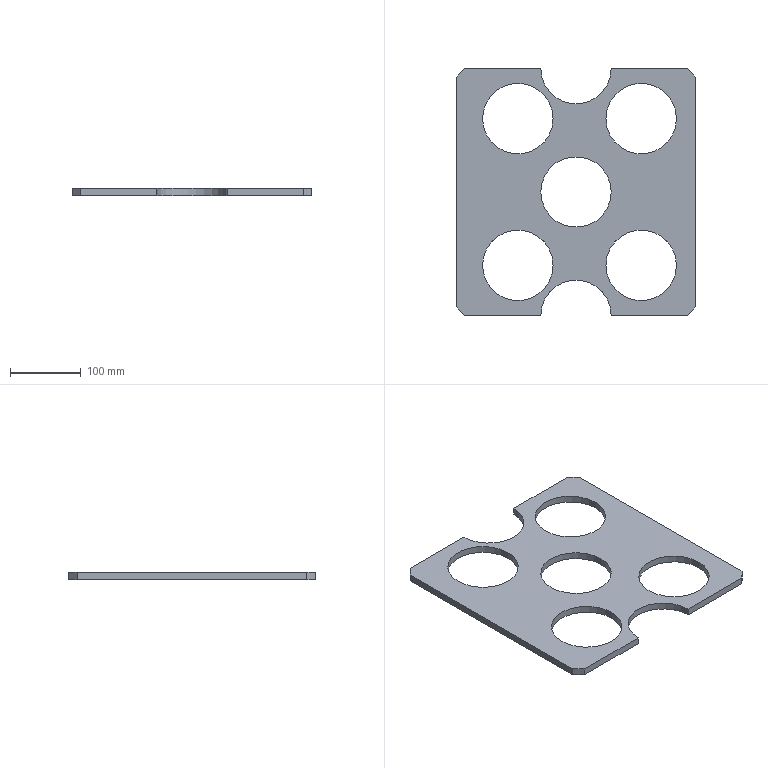Part | SolidWorks | features Extrusion 1 | 1 solid | 24 faces | box 340 x 350 x 10 mm | volume 715881 mm3 | cylinder 12 | plane 12 | commonest cylinder face diameters 100 x12
STEP:
#1=CARTESIAN_POINT('',(212.5,71.,10.));
#2=VERTEX_POINT('',#1);
#3=CARTESIAN_POINT('',(312.5,71.,10.));
#4=VERTEX_POINT('',#3);
#5=CARTESIAN_POINT('',(262.5,71.,10.));
#6=DIRECTION('',(0.,0.,1.));
#7=DIRECTION('',(-1.,0.,0.));
#8=AXIS2_PLACEMENT_3D('',#5,#6,#7);
#9=CIRCLE('',#8,50.);
#10=EDGE_CURVE('',#2,#4,#9,.T.);
#11=ORIENTED_EDGE('',*,*,#10,.T.);
#12=CARTESIAN_POINT('',(312.5,71.,0.));
#13=VERTEX_POINT('',#12);
#14=CARTESIAN_POINT('',(312.5,71.,10.));
#15=DIRECTION('',(0.,0.,-1.));
#16=VECTOR('',#15,1000.);
#17=LINE('',#14,#16);
#18=EDGE_CURVE('',#4,#13,#17,.T.);
#19=ORIENTED_EDGE('',*,*,#18,.T.);
#20=CARTESIAN_POINT('',(212.5,71.,0.));
#21=VERTEX_POINT('',#20);
#22=CARTESIAN_POINT('',(262.5,71.,0.));
#23=DIRECTION('',(0.,0.,1.));
#24=DIRECTION('',(-1.,0.,0.));
#25=AXIS2_PLACEMENT_3D('',#22,#23,#24);
#26=CIRCLE('',#25,50.);
#27=EDGE_CURVE('',#21,#13,#26,.T.);
#28=ORIENTED_EDGE('',*,*,#27,.F.);
#29=CARTESIAN_POINT('',(212.5,71.,10.));
#30=DIRECTION('',(0.,0.,-1.));
#31=VECTOR('',#30,1000.);
#32=LINE('',#29,#31);
#33=EDGE_CURVE('',#2,#21,#32,.T.);
#34=ORIENTED_EDGE('',*,*,#33,.F.);
#35=EDGE_LOOP('',(#11,#19,#28,#34));
#36=FACE_OUTER_BOUND('',#35,.T.);
#37=CARTESIAN_POINT('',(262.5,71.,10.));
#38=DIRECTION('',(0.,0.,-1.));
#39=DIRECTION('',(-1.,0.,0.));
#40=AXIS2_PLACEMENT_3D('',#37,#38,#39);
#41=CYLINDRICAL_SURFACE('',#40,50.);
#42=ADVANCED_FACE('',(#36),#41,.F.);
#43=CARTESIAN_POINT('',(37.5,71.,10.));
#44=VERTEX_POINT('',#43);
#45=CARTESIAN_POINT('',(137.5,71.,10.));
#46=VERTEX_POINT('',#45);
#47=CARTESIAN_POINT('',(87.5,71.,10.));
#48=DIRECTION('',(0.,0.,1.));
#49=DIRECTION('',(-1.,0.,0.));
#50=AXIS2_PLACEMENT_3D('',#47,#48,#49);
#51=CIRCLE('',#50,50.);
#52=EDGE_CURVE('',#44,#46,#51,.T.);
#53=ORIENTED_EDGE('',*,*,#52,.T.);
#54=CARTESIAN_POINT('',(137.5,71.,0.));
#55=VERTEX_POINT('',#54);
#56=CARTESIAN_POINT('',(137.5,71.,10.));
#57=DIRECTION('',(0.,0.,-1.));
#58=VECTOR('',#57,1000.);
#59=LINE('',#56,#58);
#60=EDGE_CURVE('',#46,#55,#59,.T.);
#61=ORIENTED_EDGE('',*,*,#60,.T.);
#62=CARTESIAN_POINT('',(37.5,71.,0.));
#63=VERTEX_POINT('',#62);
#64=CARTESIAN_POINT('',(87.5,71.,0.));
#65=DIRECTION('',(0.,0.,1.));
#66=DIRECTION('',(-1.,0.,0.));
#67=AXIS2_PLACEMENT_3D('',#64,#65,#66);
#68=CIRCLE('',#67,50.);
#69=EDGE_CURVE('',#63,#55,#68,.T.);
#70=ORIENTED_EDGE('',*,*,#69,.F.);
#71=CARTESIAN_POINT('',(37.5,71.,10.));
#72=DIRECTION('',(0.,0.,-1.));
#73=VECTOR('',#72,1000.);
#74=LINE('',#71,#73);
#75=EDGE_CURVE('',#44,#63,#74,.T.);
#76=ORIENTED_EDGE('',*,*,#75,.F.);
#77=EDGE_LOOP('',(#53,#61,#70,#76));
#78=FACE_OUTER_BOUND('',#77,.T.);
#79=CARTESIAN_POINT('',(87.5,71.,10.));
#80=DIRECTION('',(0.,0.,-1.));
#81=DIRECTION('',(-1.,0.,0.));
#82=AXIS2_PLACEMENT_3D('',#79,#80,#81);
#83=CYLINDRICAL_SURFACE('',#82,50.);
#84=ADVANCED_FACE('',(#78),#83,.F.);
#85=CARTESIAN_POINT('',(212.5,279.,10.));
#86=VERTEX_POINT('',#85);
#87=CARTESIAN_POINT('',(312.5,279.,10.));
#88=VERTEX_POINT('',#87);
#89=CARTESIAN_POINT('',(262.5,279.,10.));
#90=DIRECTION('',(0.,0.,1.));
#91=DIRECTION('',(1.,0.,0.));
#92=AXIS2_PLACEMENT_3D('',#89,#90,#91);
#93=CIRCLE('',#92,50.);
#94=EDGE_CURVE('',#86,#88,#93,.T.);
#95=ORIENTED_EDGE('',*,*,#94,.T.);
#96=CARTESIAN_POINT('',(312.5,279.,0.));
#97=VERTEX_POINT('',#96);
#98=CARTESIAN_POINT('',(312.5,279.,10.));
#99=DIRECTION('',(0.,0.,-1.));
#100=VECTOR('',#99,1000.);
#101=LINE('',#98,#100);
#102=EDGE_CURVE('',#88,#97,#101,.T.);
#103=ORIENTED_EDGE('',*,*,#102,.T.);
#104=CARTESIAN_POINT('',(212.5,279.,0.));
#105=VERTEX_POINT('',#104);
#106=CARTESIAN_POINT('',(262.5,279.,0.));
#107=DIRECTION('',(0.,0.,1.));
#108=DIRECTION('',(1.,0.,0.));
#109=AXIS2_PLACEMENT_3D('',#106,#107,#108);
#110=CIRCLE('',#109,50.);
#111=EDGE_CURVE('',#105,#97,#110,.T.);
#112=ORIENTED_EDGE('',*,*,#111,.F.);
#113=CARTESIAN_POINT('',(212.5,279.,10.));
#114=DIRECTION('',(0.,0.,-1.));
#115=VECTOR('',#114,1000.);
#116=LINE('',#113,#115);
#117=EDGE_CURVE('',#86,#105,#116,.T.);
#118=ORIENTED_EDGE('',*,*,#117,.F.);
#119=EDGE_LOOP('',(#95,#103,#112,#118));
#120=FACE_OUTER_BOUND('',#119,.T.);
#121=CARTESIAN_POINT('',(262.5,279.,10.));
#122=DIRECTION('',(0.,0.,-1.));
#123=DIRECTION('',(-1.,0.,0.));
#124=AXIS2_PLACEMENT_3D('',#121,#122,#123);
#125=CYLINDRICAL_SURFACE('',#124,50.);
#126=ADVANCED_FACE('',(#120),#125,.F.);
#127=CARTESIAN_POINT('',(37.5,279.,10.));
#128=VERTEX_POINT('',#127);
#129=CARTESIAN_POINT('',(137.5,279.,10.));
#130=VERTEX_POINT('',#129);
#131=CARTESIAN_POINT('',(87.5,279.,10.));
#132=DIRECTION('',(0.,0.,1.));
#133=DIRECTION('',(1.,0.,0.));
#134=AXIS2_PLACEMENT_3D('',#131,#132,#133);
#135=CIRCLE('',#134,50.);
#136=EDGE_CURVE('',#128,#130,#135,.T.);
#137=ORIENTED_EDGE('',*,*,#136,.T.);
#138=CARTESIAN_POINT('',(137.5,279.,0.));
#139=VERTEX_POINT('',#138);
#140=CARTESIAN_POINT('',(137.5,279.,10.));
#141=DIRECTION('',(0.,0.,-1.));
#142=VECTOR('',#141,1000.);
#143=LINE('',#140,#142);
#144=EDGE_CURVE('',#130,#139,#143,.T.);
#145=ORIENTED_EDGE('',*,*,#144,.T.);
#146=CARTESIAN_POINT('',(37.5,279.,0.));
#147=VERTEX_POINT('',#146);
#148=CARTESIAN_POINT('',(87.5,279.,0.));
#149=DIRECTION('',(0.,0.,1.));
#150=DIRECTION('',(1.,0.,0.));
#151=AXIS2_PLACEMENT_3D('',#148,#149,#150);
#152=CIRCLE('',#151,50.);
#153=EDGE_CURVE('',#147,#139,#152,.T.);
#154=ORIENTED_EDGE('',*,*,#153,.F.);
#155=CARTESIAN_POINT('',(37.5,279.,10.));
#156=DIRECTION('',(0.,0.,-1.));
#157=VECTOR('',#156,1000.);
#158=LINE('',#155,#157);
#159=EDGE_CURVE('',#128,#147,#158,.T.);
#160=ORIENTED_EDGE('',*,*,#159,.F.);
#161=EDGE_LOOP('',(#137,#145,#154,#160));
#162=FACE_OUTER_BOUND('',#161,.T.);
#163=CARTESIAN_POINT('',(87.5,279.,10.));
#164=DIRECTION('',(0.,0.,-1.));
#165=DIRECTION('',(-1.,0.,0.));
#166=AXIS2_PLACEMENT_3D('',#163,#164,#165);
#167=CYLINDRICAL_SURFACE('',#166,50.);
#168=ADVANCED_FACE('',(#162),#167,.F.);
#169=CARTESIAN_POINT('',(120.,175.,10.));
#170=VERTEX_POINT('',#169);
#171=CARTESIAN_POINT('',(220.,175.,10.));
#172=VERTEX_POINT('',#171);
#173=CARTESIAN_POINT('',(170.,175.,10.));
#174=DIRECTION('',(0.,0.,1.));
#175=DIRECTION('',(1.,0.,0.));
#176=AXIS2_PLACEMENT_3D('',#173,#174,#175);
#177=CIRCLE('',#176,50.);
#178=EDGE_CURVE('',#170,#172,#177,.T.);
#179=ORIENTED_EDGE('',*,*,#178,.T.);
#180=CARTESIAN_POINT('',(220.,175.,0.));
#181=VERTEX_POINT('',#180);
#182=CARTESIAN_POINT('',(220.,175.,10.));
#183=DIRECTION('',(0.,0.,-1.));
#184=VECTOR('',#183,1000.);
#185=LINE('',#182,#184);
#186=EDGE_CURVE('',#172,#181,#185,.T.);
#187=ORIENTED_EDGE('',*,*,#186,.T.);
#188=CARTESIAN_POINT('',(120.,175.,0.));
#189=VERTEX_POINT('',#188);
#190=CARTESIAN_POINT('',(170.,175.,0.));
#191=DIRECTION('',(0.,0.,1.));
#192=DIRECTION('',(1.,0.,0.));
#193=AXIS2_PLACEMENT_3D('',#190,#191,#192);
#194=CIRCLE('',#193,50.);
#195=EDGE_CURVE('',#189,#181,#194,.T.);
#196=ORIENTED_EDGE('',*,*,#195,.F.);
#197=CARTESIAN_POINT('',(120.,175.,10.));
#198=DIRECTION('',(0.,0.,-1.));
#199=VECTOR('',#198,1000.);
#200=LINE('',#197,#199);
#201=EDGE_CURVE('',#170,#189,#200,.T.);
#202=ORIENTED_EDGE('',*,*,#201,.F.);
#203=EDGE_LOOP('',(#179,#187,#196,#202));
#204=FACE_OUTER_BOUND('',#203,.T.);
#205=CARTESIAN_POINT('',(170.,175.,10.));
#206=DIRECTION('',(0.,0.,-1.));
#207=DIRECTION('',(-1.,0.,0.));
#208=AXIS2_PLACEMENT_3D('',#205,#206,#207);
#209=CYLINDRICAL_SURFACE('',#208,50.);
#210=ADVANCED_FACE('',(#204),#209,.F.);
#211=ORIENTED_EDGE('',*,*,#52,.F.);
#212=CARTESIAN_POINT('',(87.5,71.,10.));
#213=DIRECTION('',(0.,0.,1.));
#214=DIRECTION('',(-1.,0.,0.));
#215=AXIS2_PLACEMENT_3D('',#212,#213,#214);
#216=CIRCLE('',#215,50.);
#217=EDGE_CURVE('',#46,#44,#216,.T.);
#218=ORIENTED_EDGE('',*,*,#217,.F.);
#219=EDGE_LOOP('',(#211,#218));
#220=FACE_BOUND('',#219,.T.);
#221=ORIENTED_EDGE('',*,*,#136,.F.);
#222=CARTESIAN_POINT('',(87.5,279.,10.));
#223=DIRECTION('',(0.,0.,1.));
#224=DIRECTION('',(1.,0.,0.));
#225=AXIS2_PLACEMENT_3D('',#222,#223,#224);
#226=CIRCLE('',#225,50.);
#227=EDGE_CURVE('',#130,#128,#226,.T.);
#228=ORIENTED_EDGE('',*,*,#227,.F.);
#229=EDGE_LOOP('',(#221,#228));
#230=FACE_BOUND('',#229,.T.);
#231=CARTESIAN_POINT('',(12.,350.,10.));
#232=VERTEX_POINT('',#231);
#233=CARTESIAN_POINT('',(0.,338.,10.));
#234=VERTEX_POINT('',#233);
#235=CARTESIAN_POINT('',(0.,338.,10.));
#236=DIRECTION('',(-0.7071,-0.7071,0.));
#237=VECTOR('',#236,1000.);
#238=LINE('',#235,#237);
#239=EDGE_CURVE('',#232,#234,#238,.T.);
#240=ORIENTED_EDGE('',*,*,#239,.T.);
#241=CARTESIAN_POINT('',(0.,12.,10.));
#242=VERTEX_POINT('',#241);
#243=CARTESIAN_POINT('',(0.,12.,10.));
#244=DIRECTION('',(0.,-1.,0.));
#245=VECTOR('',#244,1000.);
#246=LINE('',#243,#245);
#247=EDGE_CURVE('',#234,#242,#246,.T.);
#248=ORIENTED_EDGE('',*,*,#247,.T.);
#249=CARTESIAN_POINT('',(12.,0.,10.));
#250=VERTEX_POINT('',#249);
#251=CARTESIAN_POINT('',(0.,12.,10.));
#252=DIRECTION('',(0.7071,-0.7071,0.));
#253=VECTOR('',#252,1000.);
#254=LINE('',#251,#253);
#255=EDGE_CURVE('',#242,#250,#254,.T.);
#256=ORIENTED_EDGE('',*,*,#255,.T.);
#257=CARTESIAN_POINT('',(120.,0.,10.));
#258=VERTEX_POINT('',#257);
#259=CARTESIAN_POINT('',(12.,0.,10.));
#260=DIRECTION('',(1.,0.,0.));
#261=VECTOR('',#260,1000.);
#262=LINE('',#259,#261);
#263=EDGE_CURVE('',#250,#258,#262,.T.);
#264=ORIENTED_EDGE('',*,*,#263,.T.);
#265=CARTESIAN_POINT('',(220.,0.,10.));
#266=VERTEX_POINT('',#265);
#267=CARTESIAN_POINT('',(170.,0.,10.));
#268=DIRECTION('',(0.,0.,-1.));
#269=DIRECTION('',(1.,0.,0.));
#270=AXIS2_PLACEMENT_3D('',#267,#268,#269);
#271=CIRCLE('',#270,50.);
#272=EDGE_CURVE('',#258,#266,#271,.T.);
#273=ORIENTED_EDGE('',*,*,#272,.T.);
#274=CARTESIAN_POINT('',(328.,0.,10.));
#275=VERTEX_POINT('',#274);
#276=CARTESIAN_POINT('',(220.,0.,10.));
#277=DIRECTION('',(1.,0.,0.));
#278=VECTOR('',#277,1000.);
#279=LINE('',#276,#278);
#280=EDGE_CURVE('',#266,#275,#279,.T.);
#281=ORIENTED_EDGE('',*,*,#280,.T.);
#282=CARTESIAN_POINT('',(340.,12.,10.));
#283=VERTEX_POINT('',#282);
#284=CARTESIAN_POINT('',(328.,0.,10.));
#285=DIRECTION('',(0.7071,0.7071,0.));
#286=VECTOR('',#285,1000.);
#287=LINE('',#284,#286);
#288=EDGE_CURVE('',#275,#283,#287,.T.);
#289=ORIENTED_EDGE('',*,*,#288,.T.);
#290=CARTESIAN_POINT('',(340.,338.,10.));
#291=VERTEX_POINT('',#290);
#292=CARTESIAN_POINT('',(340.,12.,10.));
#293=DIRECTION('',(0.,1.,0.));
#294=VECTOR('',#293,1000.);
#295=LINE('',#292,#294);
#296=EDGE_CURVE('',#283,#291,#295,.T.);
#297=ORIENTED_EDGE('',*,*,#296,.T.);
#298=CARTESIAN_POINT('',(328.,350.,10.));
#299=VERTEX_POINT('',#298);
#300=CARTESIAN_POINT('',(340.,338.,10.));
#301=DIRECTION('',(-0.7071,0.7071,0.));
#302=VECTOR('',#301,1000.);
#303=LINE('',#300,#302);
#304=EDGE_CURVE('',#291,#299,#303,.T.);
#305=ORIENTED_EDGE('',*,*,#304,.T.);
#306=CARTESIAN_POINT('',(220.,350.,10.));
#307=VERTEX_POINT('',#306);
#308=CARTESIAN_POINT('',(220.,350.,10.));
#309=DIRECTION('',(-1.,0.,0.));
#310=VECTOR('',#309,1000.);
#311=LINE('',#308,#310);
#312=EDGE_CURVE('',#299,#307,#311,.T.);
#313=ORIENTED_EDGE('',*,*,#312,.T.);
#314=CARTESIAN_POINT('',(120.,350.,10.));
#315=VERTEX_POINT('',#314);
#316=CARTESIAN_POINT('',(170.,350.,10.));
#317=DIRECTION('',(0.,0.,-1.));
#318=DIRECTION('',(1.,0.,0.));
#319=AXIS2_PLACEMENT_3D('',#316,#317,#318);
#320=CIRCLE('',#319,50.);
#321=EDGE_CURVE('',#307,#315,#320,.T.);
#322=ORIENTED_EDGE('',*,*,#321,.T.);
#323=CARTESIAN_POINT('',(12.,350.,10.));
#324=DIRECTION('',(-1.,0.,0.));
#325=VECTOR('',#324,1000.);
#326=LINE('',#323,#325);
#327=EDGE_CURVE('',#315,#232,#326,.T.);
#328=ORIENTED_EDGE('',*,*,#327,.T.);
#329=EDGE_LOOP('',(#240,#248,#256,#264,#273,#281,#289,#297,#305,#313,#322,#328));
#330=FACE_OUTER_BOUND('',#329,.T.);
#331=ORIENTED_EDGE('',*,*,#178,.F.);
#332=CARTESIAN_POINT('',(170.,175.,10.));
#333=DIRECTION('',(0.,0.,1.));
#334=DIRECTION('',(1.,0.,0.));
#335=AXIS2_PLACEMENT_3D('',#332,#333,#334);
#336=CIRCLE('',#335,50.);
#337=EDGE_CURVE('',#172,#170,#336,.T.);
#338=ORIENTED_EDGE('',*,*,#337,.F.);
#339=EDGE_LOOP('',(#331,#338));
#340=FACE_BOUND('',#339,.T.);
#341=ORIENTED_EDGE('',*,*,#94,.F.);
#342=CARTESIAN_POINT('',(262.5,279.,10.));
#343=DIRECTION('',(0.,0.,1.));
#344=DIRECTION('',(1.,0.,0.));
#345=AXIS2_PLACEMENT_3D('',#342,#343,#344);
#346=CIRCLE('',#345,50.);
#347=EDGE_CURVE('',#88,#86,#346,.T.);
#348=ORIENTED_EDGE('',*,*,#347,.F.);
#349=EDGE_LOOP('',(#341,#348));
#350=FACE_BOUND('',#349,.T.);
#351=ORIENTED_EDGE('',*,*,#10,.F.);
#352=CARTESIAN_POINT('',(262.5,71.,10.));
#353=DIRECTION('',(0.,0.,1.));
#354=DIRECTION('',(-1.,0.,0.));
#355=AXIS2_PLACEMENT_3D('',#352,#353,#354);
#356=CIRCLE('',#355,50.);
#357=EDGE_CURVE('',#4,#2,#356,.T.);
#358=ORIENTED_EDGE('',*,*,#357,.F.);
#359=EDGE_LOOP('',(#351,#358));
#360=FACE_BOUND('',#359,.T.);
#361=CARTESIAN_POINT('',(170.,350.,10.));
#362=DIRECTION('',(0.,0.,1.));
#363=DIRECTION('',(1.,0.,0.));
#364=AXIS2_PLACEMENT_3D('',#361,#362,#363);
#365=PLANE('',#364);
#366=ADVANCED_FACE('',(#220,#230,#330,#340,#350,#360),#365,.T.);
#367=ORIENTED_EDGE('',*,*,#69,.T.);
#368=CARTESIAN_POINT('',(87.5,71.,0.));
#369=DIRECTION('',(0.,0.,1.));
#370=DIRECTION('',(-1.,0.,0.));
#371=AXIS2_PLACEMENT_3D('',#368,#369,#370);
#372=CIRCLE('',#371,50.);
#373=EDGE_CURVE('',#55,#63,#372,.T.);
#374=ORIENTED_EDGE('',*,*,#373,.T.);
#375=EDGE_LOOP('',(#367,#374));
#376=FACE_BOUND('',#375,.T.);
#377=ORIENTED_EDGE('',*,*,#153,.T.);
#378=CARTESIAN_POINT('',(87.5,279.,0.));
#379=DIRECTION('',(0.,0.,1.));
#380=DIRECTION('',(1.,0.,0.));
#381=AXIS2_PLACEMENT_3D('',#378,#379,#380);
#382=CIRCLE('',#381,50.);
#383=EDGE_CURVE('',#139,#147,#382,.T.);
#384=ORIENTED_EDGE('',*,*,#383,.T.);
#385=EDGE_LOOP('',(#377,#384));
#386=FACE_BOUND('',#385,.T.);
#387=CARTESIAN_POINT('',(12.,350.,0.));
#388=VERTEX_POINT('',#387);
#389=CARTESIAN_POINT('',(0.,338.,0.));
#390=VERTEX_POINT('',#389);
#391=CARTESIAN_POINT('',(0.,338.,0.));
#392=DIRECTION('',(-0.7071,-0.7071,0.));
#393=VECTOR('',#392,1000.);
#394=LINE('',#391,#393);
#395=EDGE_CURVE('',#388,#390,#394,.T.);
#396=ORIENTED_EDGE('',*,*,#395,.F.);
#397=CARTESIAN_POINT('',(120.,350.,0.));
#398=VERTEX_POINT('',#397);
#399=CARTESIAN_POINT('',(12.,350.,0.));
#400=DIRECTION('',(-1.,0.,0.));
#401=VECTOR('',#400,1000.);
#402=LINE('',#399,#401);
#403=EDGE_CURVE('',#398,#388,#402,.T.);
#404=ORIENTED_EDGE('',*,*,#403,.F.);
#405=CARTESIAN_POINT('',(220.,350.,0.));
#406=VERTEX_POINT('',#405);
#407=CARTESIAN_POINT('',(170.,350.,0.));
#408=DIRECTION('',(0.,0.,-1.));
#409=DIRECTION('',(1.,0.,0.));
#410=AXIS2_PLACEMENT_3D('',#407,#408,#409);
#411=CIRCLE('',#410,50.);
#412=EDGE_CURVE('',#406,#398,#411,.T.);
#413=ORIENTED_EDGE('',*,*,#412,.F.);
#414=CARTESIAN_POINT('',(328.,350.,0.));
#415=VERTEX_POINT('',#414);
#416=CARTESIAN_POINT('',(220.,350.,0.));
#417=DIRECTION('',(-1.,0.,0.));
#418=VECTOR('',#417,1000.);
#419=LINE('',#416,#418);
#420=EDGE_CURVE('',#415,#406,#419,.T.);
#421=ORIENTED_EDGE('',*,*,#420,.F.);
#422=CARTESIAN_POINT('',(340.,338.,0.));
#423=VERTEX_POINT('',#422);
#424=CARTESIAN_POINT('',(340.,338.,0.));
#425=DIRECTION('',(-0.7071,0.7071,0.));
#426=VECTOR('',#425,1000.);
#427=LINE('',#424,#426);
#428=EDGE_CURVE('',#423,#415,#427,.T.);
#429=ORIENTED_EDGE('',*,*,#428,.F.);
#430=CARTESIAN_POINT('',(340.,12.,0.));
#431=VERTEX_POINT('',#430);
#432=CARTESIAN_POINT('',(340.,12.,0.));
#433=DIRECTION('',(0.,1.,0.));
#434=VECTOR('',#433,1000.);
#435=LINE('',#432,#434);
#436=EDGE_CURVE('',#431,#423,#435,.T.);
#437=ORIENTED_EDGE('',*,*,#436,.F.);
#438=CARTESIAN_POINT('',(328.,0.,0.));
#439=VERTEX_POINT('',#438);
#440=CARTESIAN_POINT('',(328.,0.,0.));
#441=DIRECTION('',(0.7071,0.7071,0.));
#442=VECTOR('',#441,1000.);
#443=LINE('',#440,#442);
#444=EDGE_CURVE('',#439,#431,#443,.T.);
#445=ORIENTED_EDGE('',*,*,#444,.F.);
#446=CARTESIAN_POINT('',(220.,0.,0.));
#447=VERTEX_POINT('',#446);
#448=CARTESIAN_POINT('',(220.,0.,0.));
#449=DIRECTION('',(1.,0.,0.));
#450=VECTOR('',#449,1000.);
#451=LINE('',#448,#450);
#452=EDGE_CURVE('',#447,#439,#451,.T.);
#453=ORIENTED_EDGE('',*,*,#452,.F.);
#454=CARTESIAN_POINT('',(120.,0.,0.));
#455=VERTEX_POINT('',#454);
#456=CARTESIAN_POINT('',(170.,0.,0.));
#457=DIRECTION('',(0.,0.,-1.));
#458=DIRECTION('',(1.,0.,0.));
#459=AXIS2_PLACEMENT_3D('',#456,#457,#458);
#460=CIRCLE('',#459,50.);
#461=EDGE_CURVE('',#455,#447,#460,.T.);
#462=ORIENTED_EDGE('',*,*,#461,.F.);
#463=CARTESIAN_POINT('',(12.,0.,0.));
#464=VERTEX_POINT('',#463);
#465=CARTESIAN_POINT('',(12.,0.,0.));
#466=DIRECTION('',(1.,0.,0.));
#467=VECTOR('',#466,1000.);
#468=LINE('',#465,#467);
#469=EDGE_CURVE('',#464,#455,#468,.T.);
#470=ORIENTED_EDGE('',*,*,#469,.F.);
#471=CARTESIAN_POINT('',(0.,12.,0.));
#472=VERTEX_POINT('',#471);
#473=CARTESIAN_POINT('',(0.,12.,0.));
#474=DIRECTION('',(0.7071,-0.7071,0.));
#475=VECTOR('',#474,1000.);
#476=LINE('',#473,#475);
#477=EDGE_CURVE('',#472,#464,#476,.T.);
#478=ORIENTED_EDGE('',*,*,#477,.F.);
#479=CARTESIAN_POINT('',(0.,12.,0.));
#480=DIRECTION('',(0.,-1.,0.));
#481=VECTOR('',#480,1000.);
#482=LINE('',#479,#481);
#483=EDGE_CURVE('',#390,#472,#482,.T.);
#484=ORIENTED_EDGE('',*,*,#483,.F.);
#485=EDGE_LOOP('',(#396,#404,#413,#421,#429,#437,#445,#453,#462,#470,#478,#484));
#486=FACE_OUTER_BOUND('',#485,.T.);
#487=ORIENTED_EDGE('',*,*,#195,.T.);
#488=CARTESIAN_POINT('',(170.,175.,0.));
#489=DIRECTION('',(0.,0.,1.));
#490=DIRECTION('',(1.,0.,0.));
#491=AXIS2_PLACEMENT_3D('',#488,#489,#490);
#492=CIRCLE('',#491,50.);
#493=EDGE_CURVE('',#181,#189,#492,.T.);
#494=ORIENTED_EDGE('',*,*,#493,.T.);
#495=EDGE_LOOP('',(#487,#494));
#496=FACE_BOUND('',#495,.T.);
#497=ORIENTED_EDGE('',*,*,#111,.T.);
#498=CARTESIAN_POINT('',(262.5,279.,0.));
#499=DIRECTION('',(0.,0.,1.));
#500=DIRECTION('',(1.,0.,0.));
#501=AXIS2_PLACEMENT_3D('',#498,#499,#500);
#502=CIRCLE('',#501,50.);
#503=EDGE_CURVE('',#97,#105,#502,.T.);
#504=ORIENTED_EDGE('',*,*,#503,.T.);
#505=EDGE_LOOP('',(#497,#504));
#506=FACE_BOUND('',#505,.T.);
#507=ORIENTED_EDGE('',*,*,#27,.T.);
#508=CARTESIAN_POINT('',(262.5,71.,0.));
#509=DIRECTION('',(0.,0.,1.));
#510=DIRECTION('',(-1.,0.,0.));
#511=AXIS2_PLACEMENT_3D('',#508,#509,#510);
#512=CIRCLE('',#511,50.);
#513=EDGE_CURVE('',#13,#21,#512,.T.);
#514=ORIENTED_EDGE('',*,*,#513,.T.);
#515=EDGE_LOOP('',(#507,#514));
#516=FACE_BOUND('',#515,.T.);
#517=CARTESIAN_POINT('',(170.,350.,0.));
#518=DIRECTION('',(0.,0.,1.));
#519=DIRECTION('',(1.,0.,0.));
#520=AXIS2_PLACEMENT_3D('',#517,#518,#519);
#521=PLANE('',#520);
#522=ADVANCED_FACE('',(#376,#386,#486,#496,#506,#516),#521,.F.);
#523=ORIENTED_EDGE('',*,*,#395,.T.);
#524=CARTESIAN_POINT('',(0.,338.,10.));
#525=DIRECTION('',(0.,0.,-1.));
#526=VECTOR('',#525,1000.);
#527=LINE('',#524,#526);
#528=EDGE_CURVE('',#234,#390,#527,.T.);
#529=ORIENTED_EDGE('',*,*,#528,.F.);
#530=ORIENTED_EDGE('',*,*,#239,.F.);
#531=CARTESIAN_POINT('',(12.,350.,10.));
#532=DIRECTION('',(0.,0.,-1.));
#533=VECTOR('',#532,1000.);
#534=LINE('',#531,#533);
#535=EDGE_CURVE('',#232,#388,#534,.T.);
#536=ORIENTED_EDGE('',*,*,#535,.T.);
#537=EDGE_LOOP('',(#523,#529,#530,#536));
#538=FACE_OUTER_BOUND('',#537,.T.);
#539=CARTESIAN_POINT('',(0.,338.,10.));
#540=DIRECTION('',(0.7071,-0.7071,0.));
#541=DIRECTION('',(0.7071,0.7071,0.));
#542=AXIS2_PLACEMENT_3D('',#539,#540,#541);
#543=PLANE('',#542);
#544=ADVANCED_FACE('',(#538),#543,.F.);
#545=ORIENTED_EDGE('',*,*,#483,.T.);
#546=CARTESIAN_POINT('',(0.,12.,10.));
#547=DIRECTION('',(0.,0.,-1.));
#548=VECTOR('',#547,1000.);
#549=LINE('',#546,#548);
#550=EDGE_CURVE('',#242,#472,#549,.T.);
#551=ORIENTED_EDGE('',*,*,#550,.F.);
#552=ORIENTED_EDGE('',*,*,#247,.F.);
#553=ORIENTED_EDGE('',*,*,#528,.T.);
#554=EDGE_LOOP('',(#545,#551,#552,#553));
#555=FACE_OUTER_BOUND('',#554,.T.);
#556=CARTESIAN_POINT('',(0.,12.,10.));
#557=DIRECTION('',(1.,0.,0.));
#558=DIRECTION('',(0.,0.,-1.));
#559=AXIS2_PLACEMENT_3D('',#556,#557,#558);
#560=PLANE('',#559);
#561=ADVANCED_FACE('',(#555),#560,.F.);
#562=ORIENTED_EDGE('',*,*,#477,.T.);
#563=CARTESIAN_POINT('',(12.,0.,10.));
#564=DIRECTION('',(0.,0.,-1.));
#565=VECTOR('',#564,1000.);
#566=LINE('',#563,#565);
#567=EDGE_CURVE('',#250,#464,#566,.T.);
#568=ORIENTED_EDGE('',*,*,#567,.F.);
#569=ORIENTED_EDGE('',*,*,#255,.F.);
#570=ORIENTED_EDGE('',*,*,#550,.T.);
#571=EDGE_LOOP('',(#562,#568,#569,#570));
#572=FACE_OUTER_BOUND('',#571,.T.);
#573=CARTESIAN_POINT('',(0.,12.,10.));
#574=DIRECTION('',(0.7071,0.7071,0.));
#575=DIRECTION('',(-0.7071,0.7071,0.));
#576=AXIS2_PLACEMENT_3D('',#573,#574,#575);
#577=PLANE('',#576);
#578=ADVANCED_FACE('',(#572),#577,.F.);
#579=ORIENTED_EDGE('',*,*,#469,.T.);
#580=CARTESIAN_POINT('',(120.,0.,10.));
#581=DIRECTION('',(0.,0.,-1.));
#582=VECTOR('',#581,1000.);
#583=LINE('',#580,#582);
#584=EDGE_CURVE('',#258,#455,#583,.T.);
#585=ORIENTED_EDGE('',*,*,#584,.F.);
#586=ORIENTED_EDGE('',*,*,#263,.F.);
#587=ORIENTED_EDGE('',*,*,#567,.T.);
#588=EDGE_LOOP('',(#579,#585,#586,#587));
#589=FACE_OUTER_BOUND('',#588,.T.);
#590=CARTESIAN_POINT('',(12.,0.,10.));
#591=DIRECTION('',(0.,1.,0.));
#592=DIRECTION('',(0.,0.,1.));
#593=AXIS2_PLACEMENT_3D('',#590,#591,#592);
#594=PLANE('',#593);
#595=ADVANCED_FACE('',(#589),#594,.F.);
#596=ORIENTED_EDGE('',*,*,#461,.T.);
#597=CARTESIAN_POINT('',(220.,0.,10.));
#598=DIRECTION('',(0.,0.,-1.));
#599=VECTOR('',#598,1000.);
#600=LINE('',#597,#599);
#601=EDGE_CURVE('',#266,#447,#600,.T.);
#602=ORIENTED_EDGE('',*,*,#601,.F.);
#603=ORIENTED_EDGE('',*,*,#272,.F.);
#604=ORIENTED_EDGE('',*,*,#584,.T.);
#605=EDGE_LOOP('',(#596,#602,#603,#604));
#606=FACE_OUTER_BOUND('',#605,.T.);
#607=CARTESIAN_POINT('',(170.,0.,10.));
#608=DIRECTION('',(0.,0.,-1.));
#609=DIRECTION('',(-1.,0.,0.));
#610=AXIS2_PLACEMENT_3D('',#607,#608,#609);
#611=CYLINDRICAL_SURFACE('',#610,50.);
#612=ADVANCED_FACE('',(#606),#611,.F.);
#613=ORIENTED_EDGE('',*,*,#452,.T.);
#614=CARTESIAN_POINT('',(328.,0.,10.));
#615=DIRECTION('',(0.,0.,-1.));
#616=VECTOR('',#615,1000.);
#617=LINE('',#614,#616);
#618=EDGE_CURVE('',#275,#439,#617,.T.);
#619=ORIENTED_EDGE('',*,*,#618,.F.);
#620=ORIENTED_EDGE('',*,*,#280,.F.);
#621=ORIENTED_EDGE('',*,*,#601,.T.);
#622=EDGE_LOOP('',(#613,#619,#620,#621));
#623=FACE_OUTER_BOUND('',#622,.T.);
#624=CARTESIAN_POINT('',(220.,0.,10.));
#625=DIRECTION('',(0.,1.,0.));
#626=DIRECTION('',(0.,0.,1.));
#627=AXIS2_PLACEMENT_3D('',#624,#625,#626);
#628=PLANE('',#627);
#629=ADVANCED_FACE('',(#623),#628,.F.);
#630=ORIENTED_EDGE('',*,*,#444,.T.);
#631=CARTESIAN_POINT('',(340.,12.,10.));
#632=DIRECTION('',(0.,0.,-1.));
#633=VECTOR('',#632,1000.);
#634=LINE('',#631,#633);
#635=EDGE_CURVE('',#283,#431,#634,.T.);
#636=ORIENTED_EDGE('',*,*,#635,.F.);
#637=ORIENTED_EDGE('',*,*,#288,.F.);
#638=ORIENTED_EDGE('',*,*,#618,.T.);
#639=EDGE_LOOP('',(#630,#636,#637,#638));
#640=FACE_OUTER_BOUND('',#639,.T.);
#641=CARTESIAN_POINT('',(328.,0.,10.));
#642=DIRECTION('',(-0.7071,0.7071,0.));
#643=DIRECTION('',(-0.7071,-0.7071,0.));
#644=AXIS2_PLACEMENT_3D('',#641,#642,#643);
#645=PLANE('',#644);
#646=ADVANCED_FACE('',(#640),#645,.F.);
#647=ORIENTED_EDGE('',*,*,#436,.T.);
#648=CARTESIAN_POINT('',(340.,338.,10.));
#649=DIRECTION('',(0.,0.,-1.));
#650=VECTOR('',#649,1000.);
#651=LINE('',#648,#650);
#652=EDGE_CURVE('',#291,#423,#651,.T.);
#653=ORIENTED_EDGE('',*,*,#652,.F.);
#654=ORIENTED_EDGE('',*,*,#296,.F.);
#655=ORIENTED_EDGE('',*,*,#635,.T.);
#656=EDGE_LOOP('',(#647,#653,#654,#655));
#657=FACE_OUTER_BOUND('',#656,.T.);
#658=CARTESIAN_POINT('',(340.,12.,10.));
#659=DIRECTION('',(-1.,0.,0.));
#660=DIRECTION('',(0.,0.,1.));
#661=AXIS2_PLACEMENT_3D('',#658,#659,#660);
#662=PLANE('',#661);
#663=ADVANCED_FACE('',(#657),#662,.F.);
#664=ORIENTED_EDGE('',*,*,#428,.T.);
#665=CARTESIAN_POINT('',(328.,350.,10.));
#666=DIRECTION('',(0.,0.,-1.));
#667=VECTOR('',#666,1000.);
#668=LINE('',#665,#667);
#669=EDGE_CURVE('',#299,#415,#668,.T.);
#670=ORIENTED_EDGE('',*,*,#669,.F.);
#671=ORIENTED_EDGE('',*,*,#304,.F.);
#672=ORIENTED_EDGE('',*,*,#652,.T.);
#673=EDGE_LOOP('',(#664,#670,#671,#672));
#674=FACE_OUTER_BOUND('',#673,.T.);
#675=CARTESIAN_POINT('',(340.,338.,10.));
#676=DIRECTION('',(-0.7071,-0.7071,0.));
#677=DIRECTION('',(0.7071,-0.7071,0.));
#678=AXIS2_PLACEMENT_3D('',#675,#676,#677);
#679=PLANE('',#678);
#680=ADVANCED_FACE('',(#674),#679,.F.);
#681=ORIENTED_EDGE('',*,*,#420,.T.);
#682=CARTESIAN_POINT('',(220.,350.,10.));
#683=DIRECTION('',(0.,0.,-1.));
#684=VECTOR('',#683,1000.);
#685=LINE('',#682,#684);
#686=EDGE_CURVE('',#307,#406,#685,.T.);
#687=ORIENTED_EDGE('',*,*,#686,.F.);
#688=ORIENTED_EDGE('',*,*,#312,.F.);
#689=ORIENTED_EDGE('',*,*,#669,.T.);
#690=EDGE_LOOP('',(#681,#687,#688,#689));
#691=FACE_OUTER_BOUND('',#690,.T.);
#692=CARTESIAN_POINT('',(220.,350.,10.));
#693=DIRECTION('',(0.,-1.,0.));
#694=DIRECTION('',(0.,0.,-1.));
#695=AXIS2_PLACEMENT_3D('',#692,#693,#694);
#696=PLANE('',#695);
#697=ADVANCED_FACE('',(#691),#696,.F.);
#698=ORIENTED_EDGE('',*,*,#412,.T.);
#699=CARTESIAN_POINT('',(120.,350.,10.));
#700=DIRECTION('',(0.,0.,-1.));
#701=VECTOR('',#700,1000.);
#702=LINE('',#699,#701);
#703=EDGE_CURVE('',#315,#398,#702,.T.);
#704=ORIENTED_EDGE('',*,*,#703,.F.);
#705=ORIENTED_EDGE('',*,*,#321,.F.);
#706=ORIENTED_EDGE('',*,*,#686,.T.);
#707=EDGE_LOOP('',(#698,#704,#705,#706));
#708=FACE_OUTER_BOUND('',#707,.T.);
#709=CARTESIAN_POINT('',(170.,350.,10.));
#710=DIRECTION('',(0.,0.,-1.));
#711=DIRECTION('',(-1.,0.,0.));
#712=AXIS2_PLACEMENT_3D('',#709,#710,#711);
#713=CYLINDRICAL_SURFACE('',#712,50.);
#714=ADVANCED_FACE('',(#708),#713,.F.);
#715=ORIENTED_EDGE('',*,*,#403,.T.);
#716=ORIENTED_EDGE('',*,*,#535,.F.);
#717=ORIENTED_EDGE('',*,*,#327,.F.);
#718=ORIENTED_EDGE('',*,*,#703,.T.);
#719=EDGE_LOOP('',(#715,#716,#717,#718));
#720=FACE_OUTER_BOUND('',#719,.T.);
#721=CARTESIAN_POINT('',(12.,350.,10.));
#722=DIRECTION('',(0.,-1.,0.));
#723=DIRECTION('',(0.,0.,-1.));
#724=AXIS2_PLACEMENT_3D('',#721,#722,#723);
#725=PLANE('',#724);
#726=ADVANCED_FACE('',(#720),#725,.F.);
#727=ORIENTED_EDGE('',*,*,#186,.F.);
#728=ORIENTED_EDGE('',*,*,#337,.T.);
#729=ORIENTED_EDGE('',*,*,#201,.T.);
#730=ORIENTED_EDGE('',*,*,#493,.F.);
#731=EDGE_LOOP('',(#727,#728,#729,#730));
#732=FACE_OUTER_BOUND('',#731,.T.);
#733=CARTESIAN_POINT('',(170.,175.,10.));
#734=DIRECTION('',(0.,0.,-1.));
#735=DIRECTION('',(-1.,0.,0.));
#736=AXIS2_PLACEMENT_3D('',#733,#734,#735);
#737=CYLINDRICAL_SURFACE('',#736,50.);
#738=ADVANCED_FACE('',(#732),#737,.F.);
#739=ORIENTED_EDGE('',*,*,#144,.F.);
#740=ORIENTED_EDGE('',*,*,#227,.T.);
#741=ORIENTED_EDGE('',*,*,#159,.T.);
#742=ORIENTED_EDGE('',*,*,#383,.F.);
#743=EDGE_LOOP('',(#739,#740,#741,#742));
#744=FACE_OUTER_BOUND('',#743,.T.);
#745=CARTESIAN_POINT('',(87.5,279.,10.));
#746=DIRECTION('',(0.,0.,-1.));
#747=DIRECTION('',(-1.,0.,0.));
#748=AXIS2_PLACEMENT_3D('',#745,#746,#747);
#749=CYLINDRICAL_SURFACE('',#748,50.);
#750=ADVANCED_FACE('',(#744),#749,.F.);
#751=ORIENTED_EDGE('',*,*,#102,.F.);
#752=ORIENTED_EDGE('',*,*,#347,.T.);
#753=ORIENTED_EDGE('',*,*,#117,.T.);
#754=ORIENTED_EDGE('',*,*,#503,.F.);
#755=EDGE_LOOP('',(#751,#752,#753,#754));
#756=FACE_OUTER_BOUND('',#755,.T.);
#757=CARTESIAN_POINT('',(262.5,279.,10.));
#758=DIRECTION('',(0.,0.,-1.));
#759=DIRECTION('',(-1.,0.,0.));
#760=AXIS2_PLACEMENT_3D('',#757,#758,#759);
#761=CYLINDRICAL_SURFACE('',#760,50.);
#762=ADVANCED_FACE('',(#756),#761,.F.);
#763=ORIENTED_EDGE('',*,*,#60,.F.);
#764=ORIENTED_EDGE('',*,*,#217,.T.);
#765=ORIENTED_EDGE('',*,*,#75,.T.);
#766=ORIENTED_EDGE('',*,*,#373,.F.);
#767=EDGE_LOOP('',(#763,#764,#765,#766));
#768=FACE_OUTER_BOUND('',#767,.T.);
#769=CARTESIAN_POINT('',(87.5,71.,10.));
#770=DIRECTION('',(0.,0.,-1.));
#771=DIRECTION('',(-1.,0.,0.));
#772=AXIS2_PLACEMENT_3D('',#769,#770,#771);
#773=CYLINDRICAL_SURFACE('',#772,50.);
#774=ADVANCED_FACE('',(#768),#773,.F.);
#775=ORIENTED_EDGE('',*,*,#18,.F.);
#776=ORIENTED_EDGE('',*,*,#357,.T.);
#777=ORIENTED_EDGE('',*,*,#33,.T.);
#778=ORIENTED_EDGE('',*,*,#513,.F.);
#779=EDGE_LOOP('',(#775,#776,#777,#778));
#780=FACE_OUTER_BOUND('',#779,.T.);
#781=CARTESIAN_POINT('',(262.5,71.,10.));
#782=DIRECTION('',(0.,0.,-1.));
#783=DIRECTION('',(-1.,0.,0.));
#784=AXIS2_PLACEMENT_3D('',#781,#782,#783);
#785=CYLINDRICAL_SURFACE('',#784,50.);
#786=ADVANCED_FACE('',(#780),#785,.F.);
#787=CLOSED_SHELL('',(#42,#84,#126,#168,#210,#366,#522,#544,#561,#578,#595,#612,#629,#646,#663,#680,#697,#714,#726,#738,#750,#762,#774,#786));
#788=MANIFOLD_SOLID_BREP('',#787);
#789=CARTESIAN_POINT('',(0.,0.,0.));
#790=DIRECTION('',(0.,0.,1.));
#791=DIRECTION('',(1.,0.,0.));
#792=AXIS2_PLACEMENT_3D('',#789,#790,#791);
#793=(LENGTH_UNIT()NAMED_UNIT(*)SI_UNIT(.MILLI.,.METRE.));
#794=UNCERTAINTY_MEASURE_WITH_UNIT(LENGTH_MEASURE(0.00001),#793,'','');
#795=(NAMED_UNIT(*)PLANE_ANGLE_UNIT()SI_UNIT($,.RADIAN.));
#796=(NAMED_UNIT(*)SI_UNIT($,.STERADIAN.)SOLID_ANGLE_UNIT());
#797=(GEOMETRIC_REPRESENTATION_CONTEXT(3)GLOBAL_UNCERTAINTY_ASSIGNED_CONTEXT((#794))GLOBAL_UNIT_ASSIGNED_CONTEXT((#793,#795,#796))REPRESENTATION_CONTEXT('',''));
#798=ADVANCED_BREP_SHAPE_REPRESENTATION('',(#788,#792),#797);